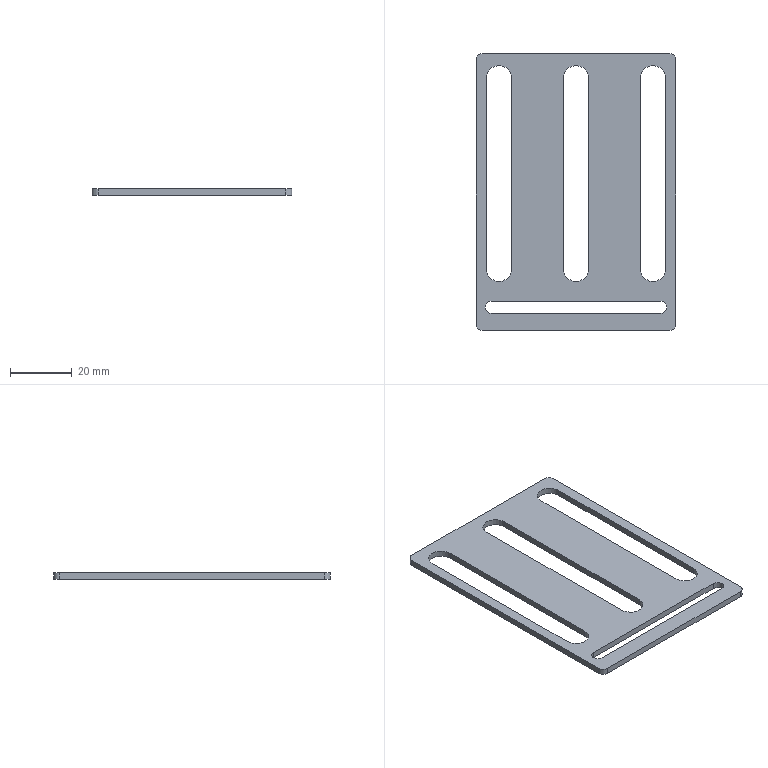Part | NX | 1 solid | 26 faces | box 65 x 90 x 2 mm | volume 7861 mm3 | plane 14 | cylinder 12 | commonest cylinder face diameters 4 x6 8.2 x6
STEP:
#1=CARTESIAN_POINT('',(32.5,-43.,-1.));
#2=VERTEX_POINT('',#1);
#3=CARTESIAN_POINT('',(32.5,43.,-1.));
#4=VERTEX_POINT('',#3);
#5=CARTESIAN_POINT('',(32.5,-45.,-1.));
#6=DIRECTION('',(0.,1.,0.));
#7=VECTOR('',#6,1000.);
#8=LINE('',#5,#7);
#9=EDGE_CURVE('',#2,#4,#8,.T.);
#10=ORIENTED_EDGE('',*,*,#9,.T.);
#11=CARTESIAN_POINT('',(32.5,43.,1.));
#12=VERTEX_POINT('',#11);
#13=CARTESIAN_POINT('',(32.5,43.,1.));
#14=DIRECTION('',(0.,0.,-1.));
#15=VECTOR('',#14,1000.);
#16=LINE('',#13,#15);
#17=EDGE_CURVE('',#4,#12,#16,.F.);
#18=ORIENTED_EDGE('',*,*,#17,.T.);
#19=CARTESIAN_POINT('',(32.5,-43.,1.));
#20=VERTEX_POINT('',#19);
#21=CARTESIAN_POINT('',(32.5,-45.,1.));
#22=DIRECTION('',(0.,1.,0.));
#23=VECTOR('',#22,1000.);
#24=LINE('',#21,#23);
#25=EDGE_CURVE('',#20,#12,#24,.T.);
#26=ORIENTED_EDGE('',*,*,#25,.F.);
#27=CARTESIAN_POINT('',(32.5,-43.,1.));
#28=DIRECTION('',(0.,0.,-1.));
#29=VECTOR('',#28,1000.);
#30=LINE('',#27,#29);
#31=EDGE_CURVE('',#20,#2,#30,.T.);
#32=ORIENTED_EDGE('',*,*,#31,.T.);
#33=EDGE_LOOP('',(#10,#18,#26,#32));
#34=FACE_BOUND('',#33,.T.);
#35=CARTESIAN_POINT('',(32.5,-45.,1.));
#36=DIRECTION('',(-1.,0.,0.));
#37=DIRECTION('',(0.,0.,1.));
#38=AXIS2_PLACEMENT_3D('',#35,#36,#37);
#39=PLANE('',#38);
#40=ADVANCED_FACE('',(#34),#39,.F.);
#41=CARTESIAN_POINT('',(30.5,45.,-1.));
#42=VERTEX_POINT('',#41);
#43=CARTESIAN_POINT('',(-30.5,45.,-1.));
#44=VERTEX_POINT('',#43);
#45=CARTESIAN_POINT('',(-32.5,45.,-1.));
#46=DIRECTION('',(-1.,0.,0.));
#47=VECTOR('',#46,1000.);
#48=LINE('',#45,#47);
#49=EDGE_CURVE('',#42,#44,#48,.T.);
#50=ORIENTED_EDGE('',*,*,#49,.T.);
#51=CARTESIAN_POINT('',(-30.5,45.,1.));
#52=VERTEX_POINT('',#51);
#53=CARTESIAN_POINT('',(-30.5,45.,1.));
#54=DIRECTION('',(0.,0.,-1.));
#55=VECTOR('',#54,1000.);
#56=LINE('',#53,#55);
#57=EDGE_CURVE('',#44,#52,#56,.F.);
#58=ORIENTED_EDGE('',*,*,#57,.T.);
#59=CARTESIAN_POINT('',(30.5,45.,1.));
#60=VERTEX_POINT('',#59);
#61=CARTESIAN_POINT('',(-32.5,45.,1.));
#62=DIRECTION('',(-1.,0.,0.));
#63=VECTOR('',#62,1000.);
#64=LINE('',#61,#63);
#65=EDGE_CURVE('',#60,#52,#64,.T.);
#66=ORIENTED_EDGE('',*,*,#65,.F.);
#67=CARTESIAN_POINT('',(30.5,45.,1.));
#68=DIRECTION('',(0.,0.,-1.));
#69=VECTOR('',#68,1000.);
#70=LINE('',#67,#69);
#71=EDGE_CURVE('',#60,#42,#70,.T.);
#72=ORIENTED_EDGE('',*,*,#71,.T.);
#73=EDGE_LOOP('',(#50,#58,#66,#72));
#74=FACE_BOUND('',#73,.T.);
#75=CARTESIAN_POINT('',(-32.5,45.,1.));
#76=DIRECTION('',(0.,-1.,0.));
#77=DIRECTION('',(0.,0.,-1.));
#78=AXIS2_PLACEMENT_3D('',#75,#76,#77);
#79=PLANE('',#78);
#80=ADVANCED_FACE('',(#74),#79,.F.);
#81=CARTESIAN_POINT('',(-32.5,43.,-1.));
#82=VERTEX_POINT('',#81);
#83=CARTESIAN_POINT('',(-32.5,-43.,-1.));
#84=VERTEX_POINT('',#83);
#85=CARTESIAN_POINT('',(-32.5,-45.,-1.));
#86=DIRECTION('',(0.,-1.,0.));
#87=VECTOR('',#86,1000.);
#88=LINE('',#85,#87);
#89=EDGE_CURVE('',#82,#84,#88,.T.);
#90=ORIENTED_EDGE('',*,*,#89,.T.);
#91=CARTESIAN_POINT('',(-32.5,-43.,1.));
#92=VERTEX_POINT('',#91);
#93=CARTESIAN_POINT('',(-32.5,-43.,1.));
#94=DIRECTION('',(0.,0.,-1.));
#95=VECTOR('',#94,1000.);
#96=LINE('',#93,#95);
#97=EDGE_CURVE('',#84,#92,#96,.F.);
#98=ORIENTED_EDGE('',*,*,#97,.T.);
#99=CARTESIAN_POINT('',(-32.5,43.,1.));
#100=VERTEX_POINT('',#99);
#101=CARTESIAN_POINT('',(-32.5,-45.,1.));
#102=DIRECTION('',(0.,-1.,0.));
#103=VECTOR('',#102,1000.);
#104=LINE('',#101,#103);
#105=EDGE_CURVE('',#100,#92,#104,.T.);
#106=ORIENTED_EDGE('',*,*,#105,.F.);
#107=CARTESIAN_POINT('',(-32.5,43.,1.));
#108=DIRECTION('',(0.,0.,-1.));
#109=VECTOR('',#108,1000.);
#110=LINE('',#107,#109);
#111=EDGE_CURVE('',#100,#82,#110,.T.);
#112=ORIENTED_EDGE('',*,*,#111,.T.);
#113=EDGE_LOOP('',(#90,#98,#106,#112));
#114=FACE_BOUND('',#113,.T.);
#115=CARTESIAN_POINT('',(-32.5,-45.,1.));
#116=DIRECTION('',(1.,0.,0.));
#117=DIRECTION('',(0.,0.,-1.));
#118=AXIS2_PLACEMENT_3D('',#115,#116,#117);
#119=PLANE('',#118);
#120=ADVANCED_FACE('',(#114),#119,.F.);
#121=CARTESIAN_POINT('',(-30.5,-45.,1.));
#122=VERTEX_POINT('',#121);
#123=CARTESIAN_POINT('',(30.5,-45.,1.));
#124=VERTEX_POINT('',#123);
#125=CARTESIAN_POINT('',(-32.5,-45.,1.));
#126=DIRECTION('',(1.,0.,0.));
#127=VECTOR('',#126,1000.);
#128=LINE('',#125,#127);
#129=EDGE_CURVE('',#122,#124,#128,.T.);
#130=ORIENTED_EDGE('',*,*,#129,.F.);
#131=CARTESIAN_POINT('',(-30.5,-45.,-1.));
#132=VERTEX_POINT('',#131);
#133=CARTESIAN_POINT('',(-30.5,-45.,1.));
#134=DIRECTION('',(0.,0.,-1.));
#135=VECTOR('',#134,1000.);
#136=LINE('',#133,#135);
#137=EDGE_CURVE('',#122,#132,#136,.T.);
#138=ORIENTED_EDGE('',*,*,#137,.T.);
#139=CARTESIAN_POINT('',(30.5,-45.,-1.));
#140=VERTEX_POINT('',#139);
#141=CARTESIAN_POINT('',(-32.5,-45.,-1.));
#142=DIRECTION('',(1.,0.,0.));
#143=VECTOR('',#142,1000.);
#144=LINE('',#141,#143);
#145=EDGE_CURVE('',#132,#140,#144,.T.);
#146=ORIENTED_EDGE('',*,*,#145,.T.);
#147=CARTESIAN_POINT('',(30.5,-45.,1.));
#148=DIRECTION('',(0.,0.,-1.));
#149=VECTOR('',#148,1000.);
#150=LINE('',#147,#149);
#151=EDGE_CURVE('',#140,#124,#150,.F.);
#152=ORIENTED_EDGE('',*,*,#151,.T.);
#153=EDGE_LOOP('',(#130,#138,#146,#152));
#154=FACE_BOUND('',#153,.T.);
#155=CARTESIAN_POINT('',(-32.5,-45.,1.));
#156=DIRECTION('',(0.,1.,0.));
#157=DIRECTION('',(0.,0.,1.));
#158=AXIS2_PLACEMENT_3D('',#155,#156,#157);
#159=PLANE('',#158);
#160=ADVANCED_FACE('',(#154),#159,.F.);
#161=CARTESIAN_POINT('',(27.5,-35.5,1.));
#162=VERTEX_POINT('',#161);
#163=CARTESIAN_POINT('',(-27.5,-35.5,1.));
#164=VERTEX_POINT('',#163);
#165=CARTESIAN_POINT('',(27.5,-35.5,1.));
#166=DIRECTION('',(-1.,0.,0.));
#167=VECTOR('',#166,1000.);
#168=LINE('',#165,#167);
#169=EDGE_CURVE('',#162,#164,#168,.T.);
#170=ORIENTED_EDGE('',*,*,#169,.F.);
#171=CARTESIAN_POINT('',(27.5,-39.5,1.));
#172=VERTEX_POINT('',#171);
#173=CARTESIAN_POINT('',(27.5,-37.5,1.));
#174=DIRECTION('',(0.,0.,1.));
#175=DIRECTION('',(1.,0.,0.));
#176=AXIS2_PLACEMENT_3D('',#173,#174,#175);
#177=CIRCLE('',#176,2.);
#178=EDGE_CURVE('',#172,#162,#177,.T.);
#179=ORIENTED_EDGE('',*,*,#178,.F.);
#180=CARTESIAN_POINT('',(-27.5,-39.5,1.));
#181=VERTEX_POINT('',#180);
#182=CARTESIAN_POINT('',(27.5,-39.5,1.));
#183=DIRECTION('',(1.,0.,0.));
#184=VECTOR('',#183,1000.);
#185=LINE('',#182,#184);
#186=EDGE_CURVE('',#181,#172,#185,.T.);
#187=ORIENTED_EDGE('',*,*,#186,.F.);
#188=CARTESIAN_POINT('',(-27.5,-37.5,1.));
#189=DIRECTION('',(0.,0.,1.));
#190=DIRECTION('',(1.,0.,0.));
#191=AXIS2_PLACEMENT_3D('',#188,#189,#190);
#192=CIRCLE('',#191,2.);
#193=EDGE_CURVE('',#164,#181,#192,.T.);
#194=ORIENTED_EDGE('',*,*,#193,.F.);
#195=EDGE_LOOP('',(#170,#179,#187,#194));
#196=FACE_BOUND('',#195,.T.);
#197=CARTESIAN_POINT('',(4.1,-25.,1.));
#198=VERTEX_POINT('',#197);
#199=CARTESIAN_POINT('',(4.1,37.,1.));
#200=VERTEX_POINT('',#199);
#201=CARTESIAN_POINT('',(4.1,-25.,1.));
#202=DIRECTION('',(0.,1.,0.));
#203=VECTOR('',#202,1000.);
#204=LINE('',#201,#203);
#205=EDGE_CURVE('',#198,#200,#204,.T.);
#206=ORIENTED_EDGE('',*,*,#205,.F.);
#207=CARTESIAN_POINT('',(-4.1,-25.,1.));
#208=VERTEX_POINT('',#207);
#209=CARTESIAN_POINT('',(0.,-25.,1.));
#210=DIRECTION('',(0.,0.,1.));
#211=DIRECTION('',(1.,0.,0.));
#212=AXIS2_PLACEMENT_3D('',#209,#210,#211);
#213=CIRCLE('',#212,4.1);
#214=EDGE_CURVE('',#208,#198,#213,.T.);
#215=ORIENTED_EDGE('',*,*,#214,.F.);
#216=CARTESIAN_POINT('',(-4.1,37.,1.));
#217=VERTEX_POINT('',#216);
#218=CARTESIAN_POINT('',(-4.1,-25.,1.));
#219=DIRECTION('',(0.,-1.,0.));
#220=VECTOR('',#219,1000.);
#221=LINE('',#218,#220);
#222=EDGE_CURVE('',#217,#208,#221,.T.);
#223=ORIENTED_EDGE('',*,*,#222,.F.);
#224=CARTESIAN_POINT('',(0.,37.,1.));
#225=DIRECTION('',(0.,0.,1.));
#226=DIRECTION('',(1.,0.,0.));
#227=AXIS2_PLACEMENT_3D('',#224,#225,#226);
#228=CIRCLE('',#227,4.1);
#229=EDGE_CURVE('',#200,#217,#228,.T.);
#230=ORIENTED_EDGE('',*,*,#229,.F.);
#231=EDGE_LOOP('',(#206,#215,#223,#230));
#232=FACE_BOUND('',#231,.T.);
#233=CARTESIAN_POINT('',(20.9,37.,1.));
#234=VERTEX_POINT('',#233);
#235=CARTESIAN_POINT('',(20.9,-25.,1.));
#236=VERTEX_POINT('',#235);
#237=CARTESIAN_POINT('',(20.9,37.,1.));
#238=DIRECTION('',(0.,-1.,0.));
#239=VECTOR('',#238,1000.);
#240=LINE('',#237,#239);
#241=EDGE_CURVE('',#234,#236,#240,.T.);
#242=ORIENTED_EDGE('',*,*,#241,.F.);
#243=CARTESIAN_POINT('',(29.1,37.,1.));
#244=VERTEX_POINT('',#243);
#245=CARTESIAN_POINT('',(25.,37.,1.));
#246=DIRECTION('',(0.,0.,1.));
#247=DIRECTION('',(-1.,0.,0.));
#248=AXIS2_PLACEMENT_3D('',#245,#246,#247);
#249=CIRCLE('',#248,4.1);
#250=EDGE_CURVE('',#244,#234,#249,.T.);
#251=ORIENTED_EDGE('',*,*,#250,.F.);
#252=CARTESIAN_POINT('',(29.1,-25.,1.));
#253=VERTEX_POINT('',#252);
#254=CARTESIAN_POINT('',(29.1,37.,1.));
#255=DIRECTION('',(0.,1.,0.));
#256=VECTOR('',#255,1000.);
#257=LINE('',#254,#256);
#258=EDGE_CURVE('',#253,#244,#257,.T.);
#259=ORIENTED_EDGE('',*,*,#258,.F.);
#260=CARTESIAN_POINT('',(25.,-25.,1.));
#261=DIRECTION('',(0.,0.,1.));
#262=DIRECTION('',(-1.,0.,0.));
#263=AXIS2_PLACEMENT_3D('',#260,#261,#262);
#264=CIRCLE('',#263,4.1);
#265=EDGE_CURVE('',#236,#253,#264,.T.);
#266=ORIENTED_EDGE('',*,*,#265,.F.);
#267=EDGE_LOOP('',(#242,#251,#259,#266));
#268=FACE_BOUND('',#267,.T.);
#269=CARTESIAN_POINT('',(-29.1,37.,1.));
#270=VERTEX_POINT('',#269);
#271=CARTESIAN_POINT('',(-29.1,-25.,1.));
#272=VERTEX_POINT('',#271);
#273=CARTESIAN_POINT('',(-29.1,37.,1.));
#274=DIRECTION('',(0.,-1.,0.));
#275=VECTOR('',#274,1000.);
#276=LINE('',#273,#275);
#277=EDGE_CURVE('',#270,#272,#276,.T.);
#278=ORIENTED_EDGE('',*,*,#277,.F.);
#279=CARTESIAN_POINT('',(-20.9,37.,1.));
#280=VERTEX_POINT('',#279);
#281=CARTESIAN_POINT('',(-25.,37.,1.));
#282=DIRECTION('',(0.,0.,1.));
#283=DIRECTION('',(1.,0.,0.));
#284=AXIS2_PLACEMENT_3D('',#281,#282,#283);
#285=CIRCLE('',#284,4.1);
#286=EDGE_CURVE('',#280,#270,#285,.T.);
#287=ORIENTED_EDGE('',*,*,#286,.F.);
#288=CARTESIAN_POINT('',(-20.9,-25.,1.));
#289=VERTEX_POINT('',#288);
#290=CARTESIAN_POINT('',(-20.9,37.,1.));
#291=DIRECTION('',(0.,1.,0.));
#292=VECTOR('',#291,1000.);
#293=LINE('',#290,#292);
#294=EDGE_CURVE('',#289,#280,#293,.T.);
#295=ORIENTED_EDGE('',*,*,#294,.F.);
#296=CARTESIAN_POINT('',(-25.,-25.,1.));
#297=DIRECTION('',(0.,0.,1.));
#298=DIRECTION('',(1.,0.,0.));
#299=AXIS2_PLACEMENT_3D('',#296,#297,#298);
#300=CIRCLE('',#299,4.1);
#301=EDGE_CURVE('',#272,#289,#300,.T.);
#302=ORIENTED_EDGE('',*,*,#301,.F.);
#303=EDGE_LOOP('',(#278,#287,#295,#302));
#304=FACE_BOUND('',#303,.T.);
#305=ORIENTED_EDGE('',*,*,#105,.T.);
#306=CARTESIAN_POINT('',(-30.5,-43.,1.));
#307=DIRECTION('',(0.,0.,-1.));
#308=DIRECTION('',(-1.,0.,0.));
#309=AXIS2_PLACEMENT_3D('',#306,#307,#308);
#310=CIRCLE('',#309,2.);
#311=EDGE_CURVE('',#92,#122,#310,.F.);
#312=ORIENTED_EDGE('',*,*,#311,.T.);
#313=ORIENTED_EDGE('',*,*,#129,.T.);
#314=CARTESIAN_POINT('',(30.5,-43.,1.));
#315=DIRECTION('',(0.,0.,-1.));
#316=DIRECTION('',(-1.,0.,0.));
#317=AXIS2_PLACEMENT_3D('',#314,#315,#316);
#318=CIRCLE('',#317,2.);
#319=EDGE_CURVE('',#124,#20,#318,.F.);
#320=ORIENTED_EDGE('',*,*,#319,.T.);
#321=ORIENTED_EDGE('',*,*,#25,.T.);
#322=CARTESIAN_POINT('',(30.5,43.,1.));
#323=DIRECTION('',(0.,0.,-1.));
#324=DIRECTION('',(-1.,0.,0.));
#325=AXIS2_PLACEMENT_3D('',#322,#323,#324);
#326=CIRCLE('',#325,2.);
#327=EDGE_CURVE('',#12,#60,#326,.F.);
#328=ORIENTED_EDGE('',*,*,#327,.T.);
#329=ORIENTED_EDGE('',*,*,#65,.T.);
#330=CARTESIAN_POINT('',(-30.5,43.,1.));
#331=DIRECTION('',(0.,0.,-1.));
#332=DIRECTION('',(-1.,0.,0.));
#333=AXIS2_PLACEMENT_3D('',#330,#331,#332);
#334=CIRCLE('',#333,2.);
#335=EDGE_CURVE('',#52,#100,#334,.F.);
#336=ORIENTED_EDGE('',*,*,#335,.T.);
#337=EDGE_LOOP('',(#305,#312,#313,#320,#321,#328,#329,#336));
#338=FACE_BOUND('',#337,.T.);
#339=CARTESIAN_POINT('',(0.,0.,1.));
#340=DIRECTION('',(0.,0.,-1.));
#341=DIRECTION('',(-1.,0.,0.));
#342=AXIS2_PLACEMENT_3D('',#339,#340,#341);
#343=PLANE('',#342);
#344=ADVANCED_FACE('',(#196,#232,#268,#304,#338),#343,.F.);
#345=CARTESIAN_POINT('',(27.5,-39.5,-1.));
#346=VERTEX_POINT('',#345);
#347=CARTESIAN_POINT('',(27.5,-35.5,-1.));
#348=VERTEX_POINT('',#347);
#349=CARTESIAN_POINT('',(27.5,-37.5,-1.));
#350=DIRECTION('',(0.,0.,1.));
#351=DIRECTION('',(1.,0.,0.));
#352=AXIS2_PLACEMENT_3D('',#349,#350,#351);
#353=CIRCLE('',#352,2.);
#354=EDGE_CURVE('',#346,#348,#353,.T.);
#355=ORIENTED_EDGE('',*,*,#354,.T.);
#356=CARTESIAN_POINT('',(-27.5,-35.5,-1.));
#357=VERTEX_POINT('',#356);
#358=CARTESIAN_POINT('',(27.5,-35.5,-1.));
#359=DIRECTION('',(-1.,0.,0.));
#360=VECTOR('',#359,1000.);
#361=LINE('',#358,#360);
#362=EDGE_CURVE('',#348,#357,#361,.T.);
#363=ORIENTED_EDGE('',*,*,#362,.T.);
#364=CARTESIAN_POINT('',(-27.5,-39.5,-1.));
#365=VERTEX_POINT('',#364);
#366=CARTESIAN_POINT('',(-27.5,-37.5,-1.));
#367=DIRECTION('',(0.,0.,1.));
#368=DIRECTION('',(1.,0.,0.));
#369=AXIS2_PLACEMENT_3D('',#366,#367,#368);
#370=CIRCLE('',#369,2.);
#371=EDGE_CURVE('',#357,#365,#370,.T.);
#372=ORIENTED_EDGE('',*,*,#371,.T.);
#373=CARTESIAN_POINT('',(27.5,-39.5,-1.));
#374=DIRECTION('',(1.,0.,0.));
#375=VECTOR('',#374,1000.);
#376=LINE('',#373,#375);
#377=EDGE_CURVE('',#365,#346,#376,.T.);
#378=ORIENTED_EDGE('',*,*,#377,.T.);
#379=EDGE_LOOP('',(#355,#363,#372,#378));
#380=FACE_BOUND('',#379,.T.);
#381=CARTESIAN_POINT('',(-4.1,-25.,-1.));
#382=VERTEX_POINT('',#381);
#383=CARTESIAN_POINT('',(4.1,-25.,-1.));
#384=VERTEX_POINT('',#383);
#385=CARTESIAN_POINT('',(0.,-25.,-1.));
#386=DIRECTION('',(0.,0.,1.));
#387=DIRECTION('',(1.,0.,0.));
#388=AXIS2_PLACEMENT_3D('',#385,#386,#387);
#389=CIRCLE('',#388,4.1);
#390=EDGE_CURVE('',#382,#384,#389,.T.);
#391=ORIENTED_EDGE('',*,*,#390,.T.);
#392=CARTESIAN_POINT('',(4.1,37.,-1.));
#393=VERTEX_POINT('',#392);
#394=CARTESIAN_POINT('',(4.1,-25.,-1.));
#395=DIRECTION('',(0.,1.,0.));
#396=VECTOR('',#395,1000.);
#397=LINE('',#394,#396);
#398=EDGE_CURVE('',#384,#393,#397,.T.);
#399=ORIENTED_EDGE('',*,*,#398,.T.);
#400=CARTESIAN_POINT('',(-4.1,37.,-1.));
#401=VERTEX_POINT('',#400);
#402=CARTESIAN_POINT('',(0.,37.,-1.));
#403=DIRECTION('',(0.,0.,1.));
#404=DIRECTION('',(1.,0.,0.));
#405=AXIS2_PLACEMENT_3D('',#402,#403,#404);
#406=CIRCLE('',#405,4.1);
#407=EDGE_CURVE('',#393,#401,#406,.T.);
#408=ORIENTED_EDGE('',*,*,#407,.T.);
#409=CARTESIAN_POINT('',(-4.1,-25.,-1.));
#410=DIRECTION('',(0.,-1.,0.));
#411=VECTOR('',#410,1000.);
#412=LINE('',#409,#411);
#413=EDGE_CURVE('',#401,#382,#412,.T.);
#414=ORIENTED_EDGE('',*,*,#413,.T.);
#415=EDGE_LOOP('',(#391,#399,#408,#414));
#416=FACE_BOUND('',#415,.T.);
#417=CARTESIAN_POINT('',(29.1,37.,-1.));
#418=VERTEX_POINT('',#417);
#419=CARTESIAN_POINT('',(20.9,37.,-1.));
#420=VERTEX_POINT('',#419);
#421=CARTESIAN_POINT('',(25.,37.,-1.));
#422=DIRECTION('',(0.,0.,1.));
#423=DIRECTION('',(-1.,0.,0.));
#424=AXIS2_PLACEMENT_3D('',#421,#422,#423);
#425=CIRCLE('',#424,4.1);
#426=EDGE_CURVE('',#418,#420,#425,.T.);
#427=ORIENTED_EDGE('',*,*,#426,.T.);
#428=CARTESIAN_POINT('',(20.9,-25.,-1.));
#429=VERTEX_POINT('',#428);
#430=CARTESIAN_POINT('',(20.9,37.,-1.));
#431=DIRECTION('',(0.,-1.,0.));
#432=VECTOR('',#431,1000.);
#433=LINE('',#430,#432);
#434=EDGE_CURVE('',#420,#429,#433,.T.);
#435=ORIENTED_EDGE('',*,*,#434,.T.);
#436=CARTESIAN_POINT('',(29.1,-25.,-1.));
#437=VERTEX_POINT('',#436);
#438=CARTESIAN_POINT('',(25.,-25.,-1.));
#439=DIRECTION('',(0.,0.,1.));
#440=DIRECTION('',(-1.,0.,0.));
#441=AXIS2_PLACEMENT_3D('',#438,#439,#440);
#442=CIRCLE('',#441,4.1);
#443=EDGE_CURVE('',#429,#437,#442,.T.);
#444=ORIENTED_EDGE('',*,*,#443,.T.);
#445=CARTESIAN_POINT('',(29.1,37.,-1.));
#446=DIRECTION('',(0.,1.,0.));
#447=VECTOR('',#446,1000.);
#448=LINE('',#445,#447);
#449=EDGE_CURVE('',#437,#418,#448,.T.);
#450=ORIENTED_EDGE('',*,*,#449,.T.);
#451=EDGE_LOOP('',(#427,#435,#444,#450));
#452=FACE_BOUND('',#451,.T.);
#453=CARTESIAN_POINT('',(-20.9,37.,-1.));
#454=VERTEX_POINT('',#453);
#455=CARTESIAN_POINT('',(-29.1,37.,-1.));
#456=VERTEX_POINT('',#455);
#457=CARTESIAN_POINT('',(-25.,37.,-1.));
#458=DIRECTION('',(0.,0.,1.));
#459=DIRECTION('',(1.,0.,0.));
#460=AXIS2_PLACEMENT_3D('',#457,#458,#459);
#461=CIRCLE('',#460,4.1);
#462=EDGE_CURVE('',#454,#456,#461,.T.);
#463=ORIENTED_EDGE('',*,*,#462,.T.);
#464=CARTESIAN_POINT('',(-29.1,-25.,-1.));
#465=VERTEX_POINT('',#464);
#466=CARTESIAN_POINT('',(-29.1,37.,-1.));
#467=DIRECTION('',(0.,-1.,0.));
#468=VECTOR('',#467,1000.);
#469=LINE('',#466,#468);
#470=EDGE_CURVE('',#456,#465,#469,.T.);
#471=ORIENTED_EDGE('',*,*,#470,.T.);
#472=CARTESIAN_POINT('',(-20.9,-25.,-1.));
#473=VERTEX_POINT('',#472);
#474=CARTESIAN_POINT('',(-25.,-25.,-1.));
#475=DIRECTION('',(0.,0.,1.));
#476=DIRECTION('',(1.,0.,0.));
#477=AXIS2_PLACEMENT_3D('',#474,#475,#476);
#478=CIRCLE('',#477,4.1);
#479=EDGE_CURVE('',#465,#473,#478,.T.);
#480=ORIENTED_EDGE('',*,*,#479,.T.);
#481=CARTESIAN_POINT('',(-20.9,37.,-1.));
#482=DIRECTION('',(0.,1.,0.));
#483=VECTOR('',#482,1000.);
#484=LINE('',#481,#483);
#485=EDGE_CURVE('',#473,#454,#484,.T.);
#486=ORIENTED_EDGE('',*,*,#485,.T.);
#487=EDGE_LOOP('',(#463,#471,#480,#486));
#488=FACE_BOUND('',#487,.T.);
#489=ORIENTED_EDGE('',*,*,#145,.F.);
#490=CARTESIAN_POINT('',(-30.5,-43.,-1.));
#491=DIRECTION('',(0.,0.,-1.));
#492=DIRECTION('',(-1.,0.,0.));
#493=AXIS2_PLACEMENT_3D('',#490,#491,#492);
#494=CIRCLE('',#493,2.);
#495=EDGE_CURVE('',#132,#84,#494,.T.);
#496=ORIENTED_EDGE('',*,*,#495,.T.);
#497=ORIENTED_EDGE('',*,*,#89,.F.);
#498=CARTESIAN_POINT('',(-30.5,43.,-1.));
#499=DIRECTION('',(0.,0.,-1.));
#500=DIRECTION('',(-1.,0.,0.));
#501=AXIS2_PLACEMENT_3D('',#498,#499,#500);
#502=CIRCLE('',#501,2.);
#503=EDGE_CURVE('',#82,#44,#502,.T.);
#504=ORIENTED_EDGE('',*,*,#503,.T.);
#505=ORIENTED_EDGE('',*,*,#49,.F.);
#506=CARTESIAN_POINT('',(30.5,43.,-1.));
#507=DIRECTION('',(0.,0.,-1.));
#508=DIRECTION('',(-1.,0.,0.));
#509=AXIS2_PLACEMENT_3D('',#506,#507,#508);
#510=CIRCLE('',#509,2.);
#511=EDGE_CURVE('',#42,#4,#510,.T.);
#512=ORIENTED_EDGE('',*,*,#511,.T.);
#513=ORIENTED_EDGE('',*,*,#9,.F.);
#514=CARTESIAN_POINT('',(30.5,-43.,-1.));
#515=DIRECTION('',(0.,0.,-1.));
#516=DIRECTION('',(-1.,0.,0.));
#517=AXIS2_PLACEMENT_3D('',#514,#515,#516);
#518=CIRCLE('',#517,2.);
#519=EDGE_CURVE('',#2,#140,#518,.T.);
#520=ORIENTED_EDGE('',*,*,#519,.T.);
#521=EDGE_LOOP('',(#489,#496,#497,#504,#505,#512,#513,#520));
#522=FACE_BOUND('',#521,.T.);
#523=CARTESIAN_POINT('',(0.,0.,-1.));
#524=DIRECTION('',(0.,0.,-1.));
#525=DIRECTION('',(-1.,0.,0.));
#526=AXIS2_PLACEMENT_3D('',#523,#524,#525);
#527=PLANE('',#526);
#528=ADVANCED_FACE('',(#380,#416,#452,#488,#522),#527,.T.);
#529=ORIENTED_EDGE('',*,*,#286,.T.);
#530=CARTESIAN_POINT('',(-29.1,37.,-1.));
#531=DIRECTION('',(0.,0.,1.));
#532=VECTOR('',#531,1000.);
#533=LINE('',#530,#532);
#534=EDGE_CURVE('',#456,#270,#533,.T.);
#535=ORIENTED_EDGE('',*,*,#534,.F.);
#536=ORIENTED_EDGE('',*,*,#462,.F.);
#537=CARTESIAN_POINT('',(-20.9,37.,-1.));
#538=DIRECTION('',(0.,0.,1.));
#539=VECTOR('',#538,1000.);
#540=LINE('',#537,#539);
#541=EDGE_CURVE('',#454,#280,#540,.T.);
#542=ORIENTED_EDGE('',*,*,#541,.T.);
#543=EDGE_LOOP('',(#529,#535,#536,#542));
#544=FACE_BOUND('',#543,.T.);
#545=CARTESIAN_POINT('',(-25.,37.,-1.));
#546=DIRECTION('',(0.,0.,1.));
#547=DIRECTION('',(1.,0.,0.));
#548=AXIS2_PLACEMENT_3D('',#545,#546,#547);
#549=CYLINDRICAL_SURFACE('',#548,4.1);
#550=ADVANCED_FACE('',(#544),#549,.F.);
#551=ORIENTED_EDGE('',*,*,#294,.T.);
#552=ORIENTED_EDGE('',*,*,#541,.F.);
#553=ORIENTED_EDGE('',*,*,#485,.F.);
#554=CARTESIAN_POINT('',(-20.9,-25.,-1.));
#555=DIRECTION('',(0.,0.,1.));
#556=VECTOR('',#555,1000.);
#557=LINE('',#554,#556);
#558=EDGE_CURVE('',#473,#289,#557,.T.);
#559=ORIENTED_EDGE('',*,*,#558,.T.);
#560=EDGE_LOOP('',(#551,#552,#553,#559));
#561=FACE_BOUND('',#560,.T.);
#562=CARTESIAN_POINT('',(-20.9,37.,-1.));
#563=DIRECTION('',(1.,0.,0.));
#564=DIRECTION('',(0.,0.,-1.));
#565=AXIS2_PLACEMENT_3D('',#562,#563,#564);
#566=PLANE('',#565);
#567=ADVANCED_FACE('',(#561),#566,.F.);
#568=ORIENTED_EDGE('',*,*,#301,.T.);
#569=ORIENTED_EDGE('',*,*,#558,.F.);
#570=ORIENTED_EDGE('',*,*,#479,.F.);
#571=CARTESIAN_POINT('',(-29.1,-25.,-1.));
#572=DIRECTION('',(0.,0.,1.));
#573=VECTOR('',#572,1000.);
#574=LINE('',#571,#573);
#575=EDGE_CURVE('',#465,#272,#574,.T.);
#576=ORIENTED_EDGE('',*,*,#575,.T.);
#577=EDGE_LOOP('',(#568,#569,#570,#576));
#578=FACE_BOUND('',#577,.T.);
#579=CARTESIAN_POINT('',(-25.,-25.,-1.));
#580=DIRECTION('',(0.,0.,1.));
#581=DIRECTION('',(1.,0.,0.));
#582=AXIS2_PLACEMENT_3D('',#579,#580,#581);
#583=CYLINDRICAL_SURFACE('',#582,4.1);
#584=ADVANCED_FACE('',(#578),#583,.F.);
#585=ORIENTED_EDGE('',*,*,#277,.T.);
#586=ORIENTED_EDGE('',*,*,#575,.F.);
#587=ORIENTED_EDGE('',*,*,#470,.F.);
#588=ORIENTED_EDGE('',*,*,#534,.T.);
#589=EDGE_LOOP('',(#585,#586,#587,#588));
#590=FACE_BOUND('',#589,.T.);
#591=CARTESIAN_POINT('',(-29.1,37.,-1.));
#592=DIRECTION('',(-1.,0.,0.));
#593=DIRECTION('',(0.,0.,1.));
#594=AXIS2_PLACEMENT_3D('',#591,#592,#593);
#595=PLANE('',#594);
#596=ADVANCED_FACE('',(#590),#595,.F.);
#597=ORIENTED_EDGE('',*,*,#250,.T.);
#598=CARTESIAN_POINT('',(20.9,37.,-1.));
#599=DIRECTION('',(0.,0.,1.));
#600=VECTOR('',#599,1000.);
#601=LINE('',#598,#600);
#602=EDGE_CURVE('',#420,#234,#601,.T.);
#603=ORIENTED_EDGE('',*,*,#602,.F.);
#604=ORIENTED_EDGE('',*,*,#426,.F.);
#605=CARTESIAN_POINT('',(29.1,37.,-1.));
#606=DIRECTION('',(0.,0.,1.));
#607=VECTOR('',#606,1000.);
#608=LINE('',#605,#607);
#609=EDGE_CURVE('',#418,#244,#608,.T.);
#610=ORIENTED_EDGE('',*,*,#609,.T.);
#611=EDGE_LOOP('',(#597,#603,#604,#610));
#612=FACE_BOUND('',#611,.T.);
#613=CARTESIAN_POINT('',(25.,37.,-1.));
#614=DIRECTION('',(0.,0.,1.));
#615=DIRECTION('',(1.,0.,0.));
#616=AXIS2_PLACEMENT_3D('',#613,#614,#615);
#617=CYLINDRICAL_SURFACE('',#616,4.1);
#618=ADVANCED_FACE('',(#612),#617,.F.);
#619=ORIENTED_EDGE('',*,*,#258,.T.);
#620=ORIENTED_EDGE('',*,*,#609,.F.);
#621=ORIENTED_EDGE('',*,*,#449,.F.);
#622=CARTESIAN_POINT('',(29.1,-25.,-1.));
#623=DIRECTION('',(0.,0.,1.));
#624=VECTOR('',#623,1000.);
#625=LINE('',#622,#624);
#626=EDGE_CURVE('',#437,#253,#625,.T.);
#627=ORIENTED_EDGE('',*,*,#626,.T.);
#628=EDGE_LOOP('',(#619,#620,#621,#627));
#629=FACE_BOUND('',#628,.T.);
#630=CARTESIAN_POINT('',(29.1,37.,-1.));
#631=DIRECTION('',(1.,0.,0.));
#632=DIRECTION('',(0.,0.,-1.));
#633=AXIS2_PLACEMENT_3D('',#630,#631,#632);
#634=PLANE('',#633);
#635=ADVANCED_FACE('',(#629),#634,.F.);
#636=ORIENTED_EDGE('',*,*,#265,.T.);
#637=ORIENTED_EDGE('',*,*,#626,.F.);
#638=ORIENTED_EDGE('',*,*,#443,.F.);
#639=CARTESIAN_POINT('',(20.9,-25.,-1.));
#640=DIRECTION('',(0.,0.,1.));
#641=VECTOR('',#640,1000.);
#642=LINE('',#639,#641);
#643=EDGE_CURVE('',#429,#236,#642,.T.);
#644=ORIENTED_EDGE('',*,*,#643,.T.);
#645=EDGE_LOOP('',(#636,#637,#638,#644));
#646=FACE_BOUND('',#645,.T.);
#647=CARTESIAN_POINT('',(25.,-25.,-1.));
#648=DIRECTION('',(0.,0.,1.));
#649=DIRECTION('',(1.,0.,0.));
#650=AXIS2_PLACEMENT_3D('',#647,#648,#649);
#651=CYLINDRICAL_SURFACE('',#650,4.1);
#652=ADVANCED_FACE('',(#646),#651,.F.);
#653=ORIENTED_EDGE('',*,*,#241,.T.);
#654=ORIENTED_EDGE('',*,*,#643,.F.);
#655=ORIENTED_EDGE('',*,*,#434,.F.);
#656=ORIENTED_EDGE('',*,*,#602,.T.);
#657=EDGE_LOOP('',(#653,#654,#655,#656));
#658=FACE_BOUND('',#657,.T.);
#659=CARTESIAN_POINT('',(20.9,37.,-1.));
#660=DIRECTION('',(-1.,0.,0.));
#661=DIRECTION('',(0.,0.,1.));
#662=AXIS2_PLACEMENT_3D('',#659,#660,#661);
#663=PLANE('',#662);
#664=ADVANCED_FACE('',(#658),#663,.F.);
#665=ORIENTED_EDGE('',*,*,#214,.T.);
#666=CARTESIAN_POINT('',(4.1,-25.,-1.));
#667=DIRECTION('',(0.,0.,1.));
#668=VECTOR('',#667,1000.);
#669=LINE('',#666,#668);
#670=EDGE_CURVE('',#384,#198,#669,.T.);
#671=ORIENTED_EDGE('',*,*,#670,.F.);
#672=ORIENTED_EDGE('',*,*,#390,.F.);
#673=CARTESIAN_POINT('',(-4.1,-25.,-1.));
#674=DIRECTION('',(0.,0.,1.));
#675=VECTOR('',#674,1000.);
#676=LINE('',#673,#675);
#677=EDGE_CURVE('',#382,#208,#676,.T.);
#678=ORIENTED_EDGE('',*,*,#677,.T.);
#679=EDGE_LOOP('',(#665,#671,#672,#678));
#680=FACE_BOUND('',#679,.T.);
#681=CARTESIAN_POINT('',(0.,-25.,-1.));
#682=DIRECTION('',(0.,0.,1.));
#683=DIRECTION('',(1.,0.,0.));
#684=AXIS2_PLACEMENT_3D('',#681,#682,#683);
#685=CYLINDRICAL_SURFACE('',#684,4.1);
#686=ADVANCED_FACE('',(#680),#685,.F.);
#687=ORIENTED_EDGE('',*,*,#222,.T.);
#688=ORIENTED_EDGE('',*,*,#677,.F.);
#689=ORIENTED_EDGE('',*,*,#413,.F.);
#690=CARTESIAN_POINT('',(-4.1,37.,-1.));
#691=DIRECTION('',(0.,0.,1.));
#692=VECTOR('',#691,1000.);
#693=LINE('',#690,#692);
#694=EDGE_CURVE('',#401,#217,#693,.T.);
#695=ORIENTED_EDGE('',*,*,#694,.T.);
#696=EDGE_LOOP('',(#687,#688,#689,#695));
#697=FACE_BOUND('',#696,.T.);
#698=CARTESIAN_POINT('',(-4.1,-25.,-1.));
#699=DIRECTION('',(-1.,0.,0.));
#700=DIRECTION('',(0.,0.,1.));
#701=AXIS2_PLACEMENT_3D('',#698,#699,#700);
#702=PLANE('',#701);
#703=ADVANCED_FACE('',(#697),#702,.F.);
#704=ORIENTED_EDGE('',*,*,#229,.T.);
#705=ORIENTED_EDGE('',*,*,#694,.F.);
#706=ORIENTED_EDGE('',*,*,#407,.F.);
#707=CARTESIAN_POINT('',(4.1,37.,-1.));
#708=DIRECTION('',(0.,0.,1.));
#709=VECTOR('',#708,1000.);
#710=LINE('',#707,#709);
#711=EDGE_CURVE('',#393,#200,#710,.T.);
#712=ORIENTED_EDGE('',*,*,#711,.T.);
#713=EDGE_LOOP('',(#704,#705,#706,#712));
#714=FACE_BOUND('',#713,.T.);
#715=CARTESIAN_POINT('',(0.,37.,-1.));
#716=DIRECTION('',(0.,0.,1.));
#717=DIRECTION('',(1.,0.,0.));
#718=AXIS2_PLACEMENT_3D('',#715,#716,#717);
#719=CYLINDRICAL_SURFACE('',#718,4.1);
#720=ADVANCED_FACE('',(#714),#719,.F.);
#721=ORIENTED_EDGE('',*,*,#205,.T.);
#722=ORIENTED_EDGE('',*,*,#711,.F.);
#723=ORIENTED_EDGE('',*,*,#398,.F.);
#724=ORIENTED_EDGE('',*,*,#670,.T.);
#725=EDGE_LOOP('',(#721,#722,#723,#724));
#726=FACE_BOUND('',#725,.T.);
#727=CARTESIAN_POINT('',(4.1,-25.,-1.));
#728=DIRECTION('',(1.,0.,0.));
#729=DIRECTION('',(0.,0.,-1.));
#730=AXIS2_PLACEMENT_3D('',#727,#728,#729);
#731=PLANE('',#730);
#732=ADVANCED_FACE('',(#726),#731,.F.);
#733=ORIENTED_EDGE('',*,*,#178,.T.);
#734=CARTESIAN_POINT('',(27.5,-35.5,-1.));
#735=DIRECTION('',(0.,0.,1.));
#736=VECTOR('',#735,1000.);
#737=LINE('',#734,#736);
#738=EDGE_CURVE('',#348,#162,#737,.T.);
#739=ORIENTED_EDGE('',*,*,#738,.F.);
#740=ORIENTED_EDGE('',*,*,#354,.F.);
#741=CARTESIAN_POINT('',(27.5,-39.5,-1.));
#742=DIRECTION('',(0.,0.,1.));
#743=VECTOR('',#742,1000.);
#744=LINE('',#741,#743);
#745=EDGE_CURVE('',#346,#172,#744,.T.);
#746=ORIENTED_EDGE('',*,*,#745,.T.);
#747=EDGE_LOOP('',(#733,#739,#740,#746));
#748=FACE_BOUND('',#747,.T.);
#749=CARTESIAN_POINT('',(27.5,-37.5,-1.));
#750=DIRECTION('',(0.,0.,1.));
#751=DIRECTION('',(1.,0.,0.));
#752=AXIS2_PLACEMENT_3D('',#749,#750,#751);
#753=CYLINDRICAL_SURFACE('',#752,2.);
#754=ADVANCED_FACE('',(#748),#753,.F.);
#755=ORIENTED_EDGE('',*,*,#186,.T.);
#756=ORIENTED_EDGE('',*,*,#745,.F.);
#757=ORIENTED_EDGE('',*,*,#377,.F.);
#758=CARTESIAN_POINT('',(-27.5,-39.5,-1.));
#759=DIRECTION('',(0.,0.,1.));
#760=VECTOR('',#759,1000.);
#761=LINE('',#758,#760);
#762=EDGE_CURVE('',#365,#181,#761,.T.);
#763=ORIENTED_EDGE('',*,*,#762,.T.);
#764=EDGE_LOOP('',(#755,#756,#757,#763));
#765=FACE_BOUND('',#764,.T.);
#766=CARTESIAN_POINT('',(27.5,-39.5,-1.));
#767=DIRECTION('',(0.,-1.,0.));
#768=DIRECTION('',(0.,0.,-1.));
#769=AXIS2_PLACEMENT_3D('',#766,#767,#768);
#770=PLANE('',#769);
#771=ADVANCED_FACE('',(#765),#770,.F.);
#772=ORIENTED_EDGE('',*,*,#193,.T.);
#773=ORIENTED_EDGE('',*,*,#762,.F.);
#774=ORIENTED_EDGE('',*,*,#371,.F.);
#775=CARTESIAN_POINT('',(-27.5,-35.5,-1.));
#776=DIRECTION('',(0.,0.,1.));
#777=VECTOR('',#776,1000.);
#778=LINE('',#775,#777);
#779=EDGE_CURVE('',#357,#164,#778,.T.);
#780=ORIENTED_EDGE('',*,*,#779,.T.);
#781=EDGE_LOOP('',(#772,#773,#774,#780));
#782=FACE_BOUND('',#781,.T.);
#783=CARTESIAN_POINT('',(-27.5,-37.5,-1.));
#784=DIRECTION('',(0.,0.,1.));
#785=DIRECTION('',(1.,0.,0.));
#786=AXIS2_PLACEMENT_3D('',#783,#784,#785);
#787=CYLINDRICAL_SURFACE('',#786,2.);
#788=ADVANCED_FACE('',(#782),#787,.F.);
#789=ORIENTED_EDGE('',*,*,#169,.T.);
#790=ORIENTED_EDGE('',*,*,#779,.F.);
#791=ORIENTED_EDGE('',*,*,#362,.F.);
#792=ORIENTED_EDGE('',*,*,#738,.T.);
#793=EDGE_LOOP('',(#789,#790,#791,#792));
#794=FACE_BOUND('',#793,.T.);
#795=CARTESIAN_POINT('',(27.5,-35.5,-1.));
#796=DIRECTION('',(0.,1.,0.));
#797=DIRECTION('',(0.,0.,1.));
#798=AXIS2_PLACEMENT_3D('',#795,#796,#797);
#799=PLANE('',#798);
#800=ADVANCED_FACE('',(#794),#799,.F.);
#801=ORIENTED_EDGE('',*,*,#311,.F.);
#802=ORIENTED_EDGE('',*,*,#97,.F.);
#803=ORIENTED_EDGE('',*,*,#495,.F.);
#804=ORIENTED_EDGE('',*,*,#137,.F.);
#805=EDGE_LOOP('',(#801,#802,#803,#804));
#806=FACE_BOUND('',#805,.T.);
#807=CARTESIAN_POINT('',(-30.5,-43.,1.));
#808=DIRECTION('',(0.,0.,-1.));
#809=DIRECTION('',(-1.,0.,0.));
#810=AXIS2_PLACEMENT_3D('',#807,#808,#809);
#811=CYLINDRICAL_SURFACE('',#810,2.);
#812=ADVANCED_FACE('',(#806),#811,.T.);
#813=ORIENTED_EDGE('',*,*,#335,.F.);
#814=ORIENTED_EDGE('',*,*,#57,.F.);
#815=ORIENTED_EDGE('',*,*,#503,.F.);
#816=ORIENTED_EDGE('',*,*,#111,.F.);
#817=EDGE_LOOP('',(#813,#814,#815,#816));
#818=FACE_BOUND('',#817,.T.);
#819=CARTESIAN_POINT('',(-30.5,43.,1.));
#820=DIRECTION('',(0.,0.,-1.));
#821=DIRECTION('',(-1.,0.,0.));
#822=AXIS2_PLACEMENT_3D('',#819,#820,#821);
#823=CYLINDRICAL_SURFACE('',#822,2.);
#824=ADVANCED_FACE('',(#818),#823,.T.);
#825=ORIENTED_EDGE('',*,*,#327,.F.);
#826=ORIENTED_EDGE('',*,*,#17,.F.);
#827=ORIENTED_EDGE('',*,*,#511,.F.);
#828=ORIENTED_EDGE('',*,*,#71,.F.);
#829=EDGE_LOOP('',(#825,#826,#827,#828));
#830=FACE_BOUND('',#829,.T.);
#831=CARTESIAN_POINT('',(30.5,43.,1.));
#832=DIRECTION('',(0.,0.,-1.));
#833=DIRECTION('',(-1.,0.,0.));
#834=AXIS2_PLACEMENT_3D('',#831,#832,#833);
#835=CYLINDRICAL_SURFACE('',#834,2.);
#836=ADVANCED_FACE('',(#830),#835,.T.);
#837=ORIENTED_EDGE('',*,*,#319,.F.);
#838=ORIENTED_EDGE('',*,*,#151,.F.);
#839=ORIENTED_EDGE('',*,*,#519,.F.);
#840=ORIENTED_EDGE('',*,*,#31,.F.);
#841=EDGE_LOOP('',(#837,#838,#839,#840));
#842=FACE_BOUND('',#841,.T.);
#843=CARTESIAN_POINT('',(30.5,-43.,1.));
#844=DIRECTION('',(0.,0.,-1.));
#845=DIRECTION('',(-1.,0.,0.));
#846=AXIS2_PLACEMENT_3D('',#843,#844,#845);
#847=CYLINDRICAL_SURFACE('',#846,2.);
#848=ADVANCED_FACE('',(#842),#847,.T.);
#849=CLOSED_SHELL('',(#40,#80,#120,#160,#344,#528,#550,#567,#584,#596,#618,#635,#652,#664,#686,#703,#720,#732,#754,#771,#788,#800,#812,#824,#836,#848));
#850=MANIFOLD_SOLID_BREP('',#849);
#851=(LENGTH_UNIT()NAMED_UNIT(*)SI_UNIT(.MILLI.,.METRE.));
#852=UNCERTAINTY_MEASURE_WITH_UNIT(LENGTH_MEASURE(0.00001),#851,'','');
#853=(NAMED_UNIT(*)PLANE_ANGLE_UNIT()SI_UNIT($,.RADIAN.));
#854=(NAMED_UNIT(*)SI_UNIT($,.STERADIAN.)SOLID_ANGLE_UNIT());
#855=(GEOMETRIC_REPRESENTATION_CONTEXT(3)GLOBAL_UNCERTAINTY_ASSIGNED_CONTEXT((#852))GLOBAL_UNIT_ASSIGNED_CONTEXT((#851,#853,#854))REPRESENTATION_CONTEXT('',''));
#856=ADVANCED_BREP_SHAPE_REPRESENTATION('',(#850),#855);